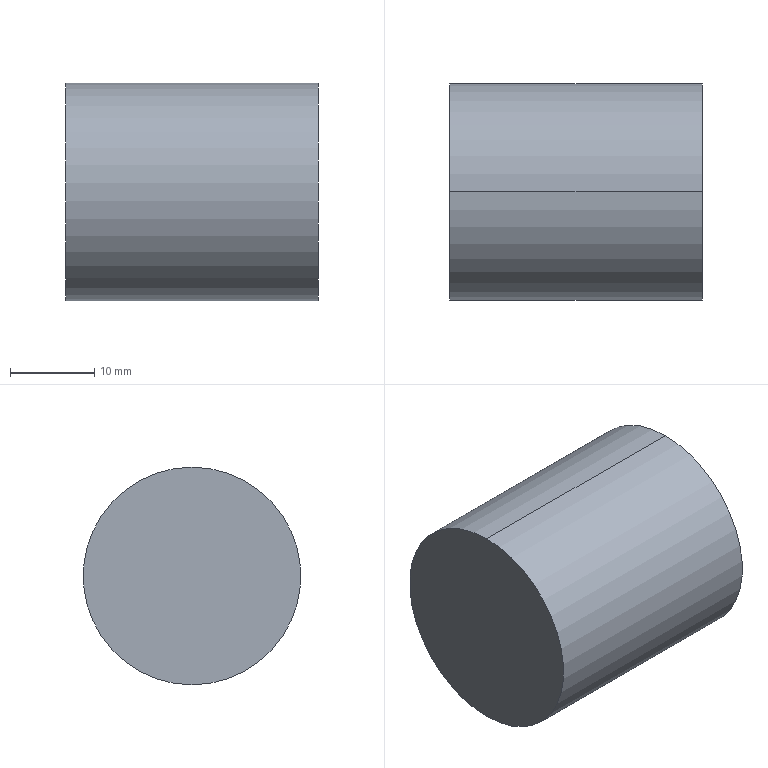Part | SolidWorks | features BaseBody 1 | 1 solid | 4 faces | box 30 x 25.832 x 25.832 mm | volume 15723 mm3 | cylinder 2 | plane 2 | commonest cylinder face diameters 25.832 x2
STEP:
#1=CARTESIAN_POINT('',(-104.,-53.,-124.084));
#2=VERTEX_POINT('',#1);
#3=CARTESIAN_POINT('',(-104.,-53.,-149.916));
#4=VERTEX_POINT('',#3);
#5=CARTESIAN_POINT('',(-104.,-53.,-137.));
#6=DIRECTION('',(-1.,0.,0.));
#7=DIRECTION('',(0.,0.,1.));
#8=AXIS2_PLACEMENT_3D('',#5,#6,#7);
#9=CIRCLE('',#8,12.916);
#10=EDGE_CURVE('',#2,#4,#9,.T.);
#11=ORIENTED_EDGE('',*,*,#10,.T.);
#12=CARTESIAN_POINT('',(-134.,-53.,-149.916));
#13=VERTEX_POINT('',#12);
#14=CARTESIAN_POINT('',(-104.,-53.,-149.916));
#15=DIRECTION('',(-1.,0.,0.));
#16=VECTOR('',#15,1000.);
#17=LINE('',#14,#16);
#18=EDGE_CURVE('',#4,#13,#17,.T.);
#19=ORIENTED_EDGE('',*,*,#18,.T.);
#20=CARTESIAN_POINT('',(-134.,-53.,-124.084));
#21=VERTEX_POINT('',#20);
#22=CARTESIAN_POINT('',(-134.,-53.,-137.));
#23=DIRECTION('',(1.,0.,0.));
#24=DIRECTION('',(0.,0.,1.));
#25=AXIS2_PLACEMENT_3D('',#22,#23,#24);
#26=CIRCLE('',#25,12.916);
#27=EDGE_CURVE('',#13,#21,#26,.T.);
#28=ORIENTED_EDGE('',*,*,#27,.T.);
#29=CARTESIAN_POINT('',(-104.,-53.,-124.084));
#30=DIRECTION('',(-1.,0.,0.));
#31=VECTOR('',#30,1000.);
#32=LINE('',#29,#31);
#33=EDGE_CURVE('',#2,#21,#32,.T.);
#34=ORIENTED_EDGE('',*,*,#33,.F.);
#35=EDGE_LOOP('',(#11,#19,#28,#34));
#36=FACE_OUTER_BOUND('',#35,.T.);
#37=CARTESIAN_POINT('',(-104.,-53.,-137.));
#38=DIRECTION('',(-1.,0.,0.));
#39=DIRECTION('',(0.,0.,1.));
#40=AXIS2_PLACEMENT_3D('',#37,#38,#39);
#41=CYLINDRICAL_SURFACE('',#40,12.916);
#42=ADVANCED_FACE('',(#36),#41,.T.);
#43=ORIENTED_EDGE('',*,*,#18,.F.);
#44=CARTESIAN_POINT('',(-104.,-53.,-137.));
#45=DIRECTION('',(-1.,0.,0.));
#46=DIRECTION('',(0.,0.,1.));
#47=AXIS2_PLACEMENT_3D('',#44,#45,#46);
#48=CIRCLE('',#47,12.916);
#49=EDGE_CURVE('',#4,#2,#48,.T.);
#50=ORIENTED_EDGE('',*,*,#49,.T.);
#51=ORIENTED_EDGE('',*,*,#33,.T.);
#52=CARTESIAN_POINT('',(-134.,-53.,-137.));
#53=DIRECTION('',(1.,0.,0.));
#54=DIRECTION('',(0.,0.,1.));
#55=AXIS2_PLACEMENT_3D('',#52,#53,#54);
#56=CIRCLE('',#55,12.916);
#57=EDGE_CURVE('',#21,#13,#56,.T.);
#58=ORIENTED_EDGE('',*,*,#57,.T.);
#59=EDGE_LOOP('',(#43,#50,#51,#58));
#60=FACE_OUTER_BOUND('',#59,.T.);
#61=CARTESIAN_POINT('',(-104.,-53.,-137.));
#62=DIRECTION('',(-1.,0.,0.));
#63=DIRECTION('',(0.,0.,1.));
#64=AXIS2_PLACEMENT_3D('',#61,#62,#63);
#65=CYLINDRICAL_SURFACE('',#64,12.916);
#66=ADVANCED_FACE('',(#60),#65,.T.);
#67=ORIENTED_EDGE('',*,*,#10,.F.);
#68=ORIENTED_EDGE('',*,*,#49,.F.);
#69=EDGE_LOOP('',(#67,#68));
#70=FACE_OUTER_BOUND('',#69,.T.);
#71=CARTESIAN_POINT('',(-104.,-53.,-137.));
#72=DIRECTION('',(1.,0.,0.));
#73=DIRECTION('',(0.,0.,-1.));
#74=AXIS2_PLACEMENT_3D('',#71,#72,#73);
#75=PLANE('',#74);
#76=ADVANCED_FACE('',(#70),#75,.T.);
#77=ORIENTED_EDGE('',*,*,#57,.F.);
#78=ORIENTED_EDGE('',*,*,#27,.F.);
#79=EDGE_LOOP('',(#77,#78));
#80=FACE_OUTER_BOUND('',#79,.T.);
#81=CARTESIAN_POINT('',(-134.,-53.,-137.));
#82=DIRECTION('',(1.,0.,0.));
#83=DIRECTION('',(0.,0.,-1.));
#84=AXIS2_PLACEMENT_3D('',#81,#82,#83);
#85=PLANE('',#84);
#86=ADVANCED_FACE('',(#80),#85,.F.);
#87=CLOSED_SHELL('',(#42,#66,#76,#86));
#88=MANIFOLD_SOLID_BREP('',#87);
#89=CARTESIAN_POINT('',(0.,0.,0.));
#90=DIRECTION('',(0.,0.,1.));
#91=DIRECTION('',(1.,0.,0.));
#92=AXIS2_PLACEMENT_3D('',#89,#90,#91);
#93=(LENGTH_UNIT()NAMED_UNIT(*)SI_UNIT(.MILLI.,.METRE.));
#94=UNCERTAINTY_MEASURE_WITH_UNIT(LENGTH_MEASURE(0.00001),#93,'','');
#95=(NAMED_UNIT(*)PLANE_ANGLE_UNIT()SI_UNIT($,.RADIAN.));
#96=(NAMED_UNIT(*)SI_UNIT($,.STERADIAN.)SOLID_ANGLE_UNIT());
#97=(GEOMETRIC_REPRESENTATION_CONTEXT(3)GLOBAL_UNCERTAINTY_ASSIGNED_CONTEXT((#94))GLOBAL_UNIT_ASSIGNED_CONTEXT((#93,#95,#96))REPRESENTATION_CONTEXT('',''));
#98=ADVANCED_BREP_SHAPE_REPRESENTATION('',(#88,#92),#97);